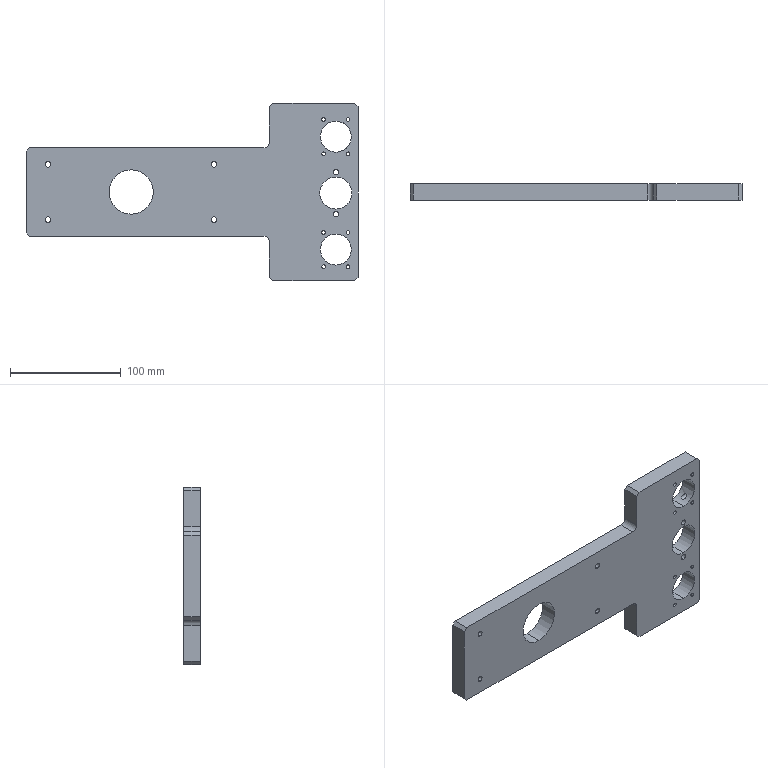Part | SolidWorks | features HoleWzd 4, ICE 3, Chamfer 2, Cut 1, Extrusion 1, Fillet 1 | 1 solid | 61 faces | box 300 x 15 x 160 mm | volume 405397 mm3 | cylinder 42 | plane 16 | cone 3 | commonest cylinder face diameters 3.3 x16 5 x12 4.2 x4 28 x4 10 x2 29 x2